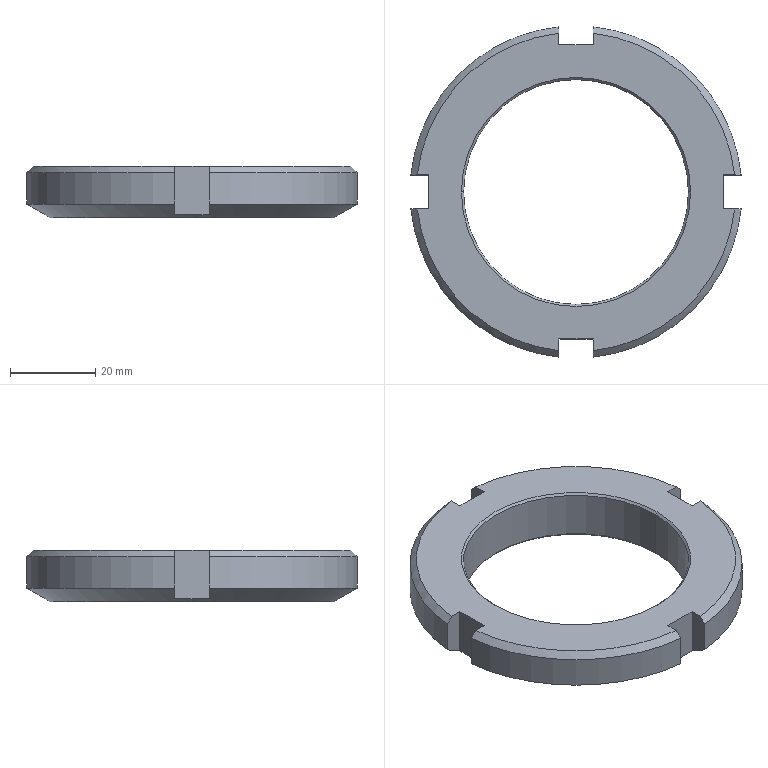Part | SolidWorks | features Chamfer 3, CirPattern 1, Cut 1, Extrusion 1 | 1 solid | 30 faces | box 77.589 x 77.589 x 12 mm | volume 27297 mm3 | plane 14 | cone 10 | cylinder 6 | commonest cylinder face diameters 78 x4 52.835 x2
STEP:
#1=CARTESIAN_POINT('',(-26.418,0.,11.5));
#2=VERTEX_POINT('',#1);
#3=CARTESIAN_POINT('',(26.418,0.,11.5));
#4=VERTEX_POINT('',#3);
#5=CARTESIAN_POINT('',(0.,0.,11.5));
#6=DIRECTION('',(0.,0.,1.));
#7=DIRECTION('',(1.,0.,0.));
#8=AXIS2_PLACEMENT_3D('',#5,#6,#7);
#9=CIRCLE('',#8,26.418);
#10=EDGE_CURVE('',#2,#4,#9,.T.);
#11=ORIENTED_EDGE('',*,*,#10,.F.);
#12=CARTESIAN_POINT('',(-26.918,0.,12.));
#13=VERTEX_POINT('',#12);
#14=CARTESIAN_POINT('',(-26.418,0.,11.5));
#15=DIRECTION('',(-0.7071,0.,0.7071));
#16=VECTOR('',#15,1000.);
#17=LINE('',#14,#16);
#18=EDGE_CURVE('',#2,#13,#17,.T.);
#19=ORIENTED_EDGE('',*,*,#18,.T.);
#20=CARTESIAN_POINT('',(26.918,0.,12.));
#21=VERTEX_POINT('',#20);
#22=CARTESIAN_POINT('',(0.,0.,12.));
#23=DIRECTION('',(0.,0.,-1.));
#24=DIRECTION('',(1.,0.,0.));
#25=AXIS2_PLACEMENT_3D('',#22,#23,#24);
#26=CIRCLE('',#25,26.918);
#27=EDGE_CURVE('',#21,#13,#26,.T.);
#28=ORIENTED_EDGE('',*,*,#27,.F.);
#29=CARTESIAN_POINT('',(26.418,0.,11.5));
#30=DIRECTION('',(0.7071,0.,0.7071));
#31=VECTOR('',#30,1000.);
#32=LINE('',#29,#31);
#33=EDGE_CURVE('',#4,#21,#32,.T.);
#34=ORIENTED_EDGE('',*,*,#33,.F.);
#35=EDGE_LOOP('',(#11,#19,#28,#34));
#36=FACE_OUTER_BOUND('',#35,.T.);
#37=CARTESIAN_POINT('',(0.,0.,11.5));
#38=DIRECTION('',(0.,0.,1.));
#39=DIRECTION('',(1.,0.,0.));
#40=AXIS2_PLACEMENT_3D('',#37,#38,#39);
#41=CONICAL_SURFACE('',#40,26.418,0.7854);
#42=ADVANCED_FACE('',(#36),#41,.F.);
#43=CARTESIAN_POINT('',(26.418,0.,0.5));
#44=VERTEX_POINT('',#43);
#45=CARTESIAN_POINT('',(-26.418,0.,0.5));
#46=VERTEX_POINT('',#45);
#47=CARTESIAN_POINT('',(0.,0.,0.5));
#48=DIRECTION('',(0.,0.,-1.));
#49=DIRECTION('',(1.,0.,0.));
#50=AXIS2_PLACEMENT_3D('',#47,#48,#49);
#51=CIRCLE('',#50,26.418);
#52=EDGE_CURVE('',#44,#46,#51,.T.);
#53=ORIENTED_EDGE('',*,*,#52,.F.);
#54=CARTESIAN_POINT('',(26.917,0.,0.));
#55=VERTEX_POINT('',#54);
#56=CARTESIAN_POINT('',(26.917,0.,0.));
#57=DIRECTION('',(0.7071,0.,-0.7071));
#58=VECTOR('',#57,1000.);
#59=LINE('',#56,#58);
#60=EDGE_CURVE('',#44,#55,#59,.T.);
#61=ORIENTED_EDGE('',*,*,#60,.T.);
#62=CARTESIAN_POINT('',(-26.917,0.,0.));
#63=VERTEX_POINT('',#62);
#64=CARTESIAN_POINT('',(0.,0.,0.));
#65=DIRECTION('',(0.,0.,1.));
#66=DIRECTION('',(1.,0.,0.));
#67=AXIS2_PLACEMENT_3D('',#64,#65,#66);
#68=CIRCLE('',#67,26.917);
#69=EDGE_CURVE('',#63,#55,#68,.T.);
#70=ORIENTED_EDGE('',*,*,#69,.F.);
#71=CARTESIAN_POINT('',(-26.917,0.,0.));
#72=DIRECTION('',(-0.7071,0.,-0.7071));
#73=VECTOR('',#72,1000.);
#74=LINE('',#71,#73);
#75=EDGE_CURVE('',#46,#63,#74,.T.);
#76=ORIENTED_EDGE('',*,*,#75,.F.);
#77=EDGE_LOOP('',(#53,#61,#70,#76));
#78=FACE_OUTER_BOUND('',#77,.T.);
#79=CARTESIAN_POINT('',(0.,0.,0.));
#80=DIRECTION('',(0.,0.,-1.));
#81=DIRECTION('',(-1.,0.,0.));
#82=AXIS2_PLACEMENT_3D('',#79,#80,#81);
#83=CONICAL_SURFACE('',#82,26.917,0.7854);
#84=ADVANCED_FACE('',(#78),#83,.F.);
#85=CARTESIAN_POINT('',(-33.5,0.,0.));
#86=VERTEX_POINT('',#85);
#87=CARTESIAN_POINT('',(33.5,0.,0.));
#88=VERTEX_POINT('',#87);
#89=CARTESIAN_POINT('',(0.,0.,0.));
#90=DIRECTION('',(0.,0.,-1.));
#91=DIRECTION('',(1.,0.,0.));
#92=AXIS2_PLACEMENT_3D('',#89,#90,#91);
#93=CIRCLE('',#92,33.5);
#94=EDGE_CURVE('',#86,#88,#93,.T.);
#95=ORIENTED_EDGE('',*,*,#94,.F.);
#96=CARTESIAN_POINT('',(-34.544,0.,0.6029));
#97=VERTEX_POINT('',#96);
#98=CARTESIAN_POINT('',(-39.,0.,3.175));
#99=DIRECTION('',(-0.866,0.,0.5));
#100=VECTOR('',#99,1000.);
#101=LINE('',#98,#100);
#102=EDGE_CURVE('',#86,#97,#101,.T.);
#103=ORIENTED_EDGE('',*,*,#102,.T.);
#104=CARTESIAN_POINT('',(-34.544,4.,0.7362));
#105=VERTEX_POINT('',#104);
#106=CARTESIAN_POINT('',(-34.544,4.,0.7362));
#107=CARTESIAN_POINT('',(-34.544,2.671,0.6479));
#108=CARTESIAN_POINT('',(-34.544,1.337,0.6029));
#109=CARTESIAN_POINT('',(-34.544,0.,0.6029));
#110=B_SPLINE_CURVE_WITH_KNOTS('',3,(#106,#107,#108,#109),.UNSPECIFIED.,.F.,.F.,(4,4),(0.01042,0.01441),.UNSPECIFIED.);
#111=EDGE_CURVE('',#105,#97,#110,.T.);
#112=ORIENTED_EDGE('',*,*,#111,.F.);
#113=CARTESIAN_POINT('',(-38.794,4.,3.175));
#114=VERTEX_POINT('',#113);
#115=CARTESIAN_POINT('',(-38.794,4.,3.175));
#116=CARTESIAN_POINT('',(-38.547,4.,3.033));
#117=CARTESIAN_POINT('',(-38.299,4.,2.891));
#118=CARTESIAN_POINT('',(-38.052,4.,2.749));
#119=CARTESIAN_POINT('',(-36.883,4.,2.078));
#120=CARTESIAN_POINT('',(-35.714,4.,1.407));
#121=CARTESIAN_POINT('',(-34.544,4.,0.7362));
#122=B_SPLINE_CURVE_WITH_KNOTS('',3,(#115,#116,#117,#118,#119,#120,#121),.UNSPECIFIED.,.F.,.F.,(4,3,4),(0.009232,0.01009,0.01413),.UNSPECIFIED.);
#123=EDGE_CURVE('',#114,#105,#122,.T.);
#124=ORIENTED_EDGE('',*,*,#123,.F.);
#125=CARTESIAN_POINT('',(-4.,38.794,3.175));
#126=VERTEX_POINT('',#125);
#127=CARTESIAN_POINT('',(0.,0.,3.175));
#128=DIRECTION('',(0.,0.,1.));
#129=DIRECTION('',(1.,0.,0.));
#130=AXIS2_PLACEMENT_3D('',#127,#128,#129);
#131=CIRCLE('',#130,39.);
#132=EDGE_CURVE('',#126,#114,#131,.T.);
#133=ORIENTED_EDGE('',*,*,#132,.F.);
#134=CARTESIAN_POINT('',(-4.,34.544,0.7362));
#135=VERTEX_POINT('',#134);
#136=CARTESIAN_POINT('',(-4.,34.544,0.7362));
#137=CARTESIAN_POINT('',(-4.,35.961,1.549));
#138=CARTESIAN_POINT('',(-4.,37.378,2.362));
#139=CARTESIAN_POINT('',(-4.,38.794,3.175));
#140=B_SPLINE_CURVE_WITH_KNOTS('',3,(#136,#137,#138,#139),.UNSPECIFIED.,.F.,.F.,(4,4),(0.009598,0.0145),.UNSPECIFIED.);
#141=EDGE_CURVE('',#135,#126,#140,.T.);
#142=ORIENTED_EDGE('',*,*,#141,.F.);
#143=CARTESIAN_POINT('',(4.,34.544,0.7362));
#144=VERTEX_POINT('',#143);
#145=CARTESIAN_POINT('',(4.,34.544,0.7362));
#146=CARTESIAN_POINT('',(2.674,34.544,0.6482));
#147=CARTESIAN_POINT('',(1.345,34.544,0.6032));
#148=CARTESIAN_POINT('',(-0.6558,34.544,0.6028));
#149=CARTESIAN_POINT('',(-1.324,34.544,0.6139));
#150=CARTESIAN_POINT('',(-2.661,34.544,0.6583));
#151=CARTESIAN_POINT('',(-3.332,34.544,0.6918));
#152=CARTESIAN_POINT('',(-4.,34.544,0.7362));
#153=B_SPLINE_CURVE_WITH_KNOTS('',3,(#145,#146,#147,#148,#149,#150,#151,#152),.UNSPECIFIED.,.F.,.F.,(4,2,2,4),(0.01042,0.0144,0.01639,0.01839),.UNSPECIFIED.);
#154=EDGE_CURVE('',#144,#135,#153,.T.);
#155=ORIENTED_EDGE('',*,*,#154,.F.);
#156=CARTESIAN_POINT('',(4.,38.794,3.175));
#157=VERTEX_POINT('',#156);
#158=CARTESIAN_POINT('',(4.,38.794,3.175));
#159=CARTESIAN_POINT('',(4.,37.378,2.362));
#160=CARTESIAN_POINT('',(4.,35.961,1.549));
#161=CARTESIAN_POINT('',(4.,34.544,0.7362));
#162=B_SPLINE_CURVE_WITH_KNOTS('',3,(#158,#159,#160,#161),.UNSPECIFIED.,.F.,.F.,(4,4),(0.005677,0.01058),.UNSPECIFIED.);
#163=EDGE_CURVE('',#157,#144,#162,.T.);
#164=ORIENTED_EDGE('',*,*,#163,.F.);
#165=CARTESIAN_POINT('',(38.794,4.,3.175));
#166=VERTEX_POINT('',#165);
#167=CARTESIAN_POINT('',(0.,0.,3.175));
#168=DIRECTION('',(0.,0.,1.));
#169=DIRECTION('',(1.,0.,0.));
#170=AXIS2_PLACEMENT_3D('',#167,#168,#169);
#171=CIRCLE('',#170,39.);
#172=EDGE_CURVE('',#166,#157,#171,.T.);
#173=ORIENTED_EDGE('',*,*,#172,.F.);
#174=CARTESIAN_POINT('',(34.544,4.,0.7362));
#175=VERTEX_POINT('',#174);
#176=CARTESIAN_POINT('',(34.544,4.,0.7362));
#177=CARTESIAN_POINT('',(35.961,4.,1.549));
#178=CARTESIAN_POINT('',(37.378,4.,2.362));
#179=CARTESIAN_POINT('',(38.794,4.,3.175));
#180=B_SPLINE_CURVE_WITH_KNOTS('',3,(#176,#177,#178,#179),.UNSPECIFIED.,.F.,.F.,(4,4),(0.009598,0.0145),.UNSPECIFIED.);
#181=EDGE_CURVE('',#175,#166,#180,.T.);
#182=ORIENTED_EDGE('',*,*,#181,.F.);
#183=CARTESIAN_POINT('',(34.544,0.,0.6029));
#184=VERTEX_POINT('',#183);
#185=CARTESIAN_POINT('',(34.544,0.,0.6029));
#186=CARTESIAN_POINT('',(34.544,1.337,0.6029));
#187=CARTESIAN_POINT('',(34.544,2.671,0.6479));
#188=CARTESIAN_POINT('',(34.544,4.,0.7362));
#189=B_SPLINE_CURVE_WITH_KNOTS('',3,(#185,#186,#187,#188),.UNSPECIFIED.,.F.,.F.,(4,4),(0.02044,0.02444),.UNSPECIFIED.);
#190=EDGE_CURVE('',#184,#175,#189,.T.);
#191=ORIENTED_EDGE('',*,*,#190,.F.);
#192=CARTESIAN_POINT('',(39.,0.,3.175));
#193=DIRECTION('',(0.866,0.,0.5));
#194=VECTOR('',#193,1000.);
#195=LINE('',#192,#194);
#196=EDGE_CURVE('',#88,#184,#195,.T.);
#197=ORIENTED_EDGE('',*,*,#196,.F.);
#198=EDGE_LOOP('',(#95,#103,#112,#124,#133,#142,#155,#164,#173,#182,#191,#197));
#199=FACE_OUTER_BOUND('',#198,.T.);
#200=CARTESIAN_POINT('',(0.,0.,3.175));
#201=DIRECTION('',(0.,0.,1.));
#202=DIRECTION('',(1.,0.,0.));
#203=AXIS2_PLACEMENT_3D('',#200,#201,#202);
#204=CONICAL_SURFACE('',#203,39.,1.047);
#205=ADVANCED_FACE('',(#199),#204,.T.);
#206=ORIENTED_EDGE('',*,*,#10,.T.);
#207=CARTESIAN_POINT('',(26.418,0.,12.));
#208=DIRECTION('',(0.,0.,-1.));
#209=VECTOR('',#208,1000.);
#210=LINE('',#207,#209);
#211=EDGE_CURVE('',#4,#44,#210,.T.);
#212=ORIENTED_EDGE('',*,*,#211,.T.);
#213=ORIENTED_EDGE('',*,*,#52,.T.);
#214=CARTESIAN_POINT('',(-26.418,0.,12.));
#215=DIRECTION('',(0.,0.,-1.));
#216=VECTOR('',#215,1000.);
#217=LINE('',#214,#216);
#218=EDGE_CURVE('',#2,#46,#217,.T.);
#219=ORIENTED_EDGE('',*,*,#218,.F.);
#220=EDGE_LOOP('',(#206,#212,#213,#219));
#221=FACE_OUTER_BOUND('',#220,.T.);
#222=CARTESIAN_POINT('',(0.,0.,12.));
#223=DIRECTION('',(0.,0.,-1.));
#224=DIRECTION('',(-1.,0.,0.));
#225=AXIS2_PLACEMENT_3D('',#222,#223,#224);
#226=CYLINDRICAL_SURFACE('',#225,26.418);
#227=ADVANCED_FACE('',(#221),#226,.F.);
#228=CARTESIAN_POINT('',(4.,38.794,10.5));
#229=VERTEX_POINT('',#228);
#230=CARTESIAN_POINT('',(38.794,4.,10.5));
#231=VERTEX_POINT('',#230);
#232=CARTESIAN_POINT('',(0.,0.,10.5));
#233=DIRECTION('',(0.,0.,-1.));
#234=DIRECTION('',(1.,0.,0.));
#235=AXIS2_PLACEMENT_3D('',#232,#233,#234);
#236=CIRCLE('',#235,39.);
#237=EDGE_CURVE('',#229,#231,#236,.T.);
#238=ORIENTED_EDGE('',*,*,#237,.T.);
#239=CARTESIAN_POINT('',(38.794,4.,0.));
#240=DIRECTION('',(0.,0.,1.));
#241=VECTOR('',#240,1000.);
#242=LINE('',#239,#241);
#243=EDGE_CURVE('',#166,#231,#242,.T.);
#244=ORIENTED_EDGE('',*,*,#243,.F.);
#245=ORIENTED_EDGE('',*,*,#172,.T.);
#246=CARTESIAN_POINT('',(4.,38.794,0.));
#247=DIRECTION('',(0.,0.,1.));
#248=VECTOR('',#247,1000.);
#249=LINE('',#246,#248);
#250=EDGE_CURVE('',#157,#229,#249,.T.);
#251=ORIENTED_EDGE('',*,*,#250,.T.);
#252=EDGE_LOOP('',(#238,#244,#245,#251));
#253=FACE_OUTER_BOUND('',#252,.T.);
#254=CARTESIAN_POINT('',(0.,0.,12.));
#255=DIRECTION('',(0.,0.,-1.));
#256=DIRECTION('',(-1.,0.,0.));
#257=AXIS2_PLACEMENT_3D('',#254,#255,#256);
#258=CYLINDRICAL_SURFACE('',#257,39.);
#259=ADVANCED_FACE('',(#253),#258,.T.);
#260=CARTESIAN_POINT('',(37.286,4.,12.));
#261=VERTEX_POINT('',#260);
#262=CARTESIAN_POINT('',(38.794,4.,10.5));
#263=CARTESIAN_POINT('',(38.402,4.,10.89));
#264=CARTESIAN_POINT('',(38.01,4.,11.28));
#265=CARTESIAN_POINT('',(37.618,4.,11.67));
#266=CARTESIAN_POINT('',(37.507,4.,11.78));
#267=CARTESIAN_POINT('',(37.397,4.,11.89));
#268=CARTESIAN_POINT('',(37.286,4.,12.));
#269=B_SPLINE_CURVE_WITH_KNOTS('',3,(#262,#263,#264,#265,#266,#267,#268),.UNSPECIFIED.,.F.,.F.,(4,3,4),(0.007216,0.008875,0.009344),.UNSPECIFIED.);
#270=EDGE_CURVE('',#231,#261,#269,.T.);
#271=ORIENTED_EDGE('',*,*,#270,.F.);
#272=ORIENTED_EDGE('',*,*,#237,.F.);
#273=CARTESIAN_POINT('',(4.,37.286,12.));
#274=VERTEX_POINT('',#273);
#275=CARTESIAN_POINT('',(4.,37.286,12.));
#276=CARTESIAN_POINT('',(4.,37.397,11.89));
#277=CARTESIAN_POINT('',(4.,37.507,11.78));
#278=CARTESIAN_POINT('',(4.,37.618,11.67));
#279=CARTESIAN_POINT('',(4.,38.01,11.28));
#280=CARTESIAN_POINT('',(4.,38.402,10.89));
#281=CARTESIAN_POINT('',(4.,38.794,10.5));
#282=B_SPLINE_CURVE_WITH_KNOTS('',3,(#275,#276,#277,#278,#279,#280,#281),.UNSPECIFIED.,.F.,.F.,(4,3,4),(0.008407,0.008875,0.01053),.UNSPECIFIED.);
#283=EDGE_CURVE('',#274,#229,#282,.T.);
#284=ORIENTED_EDGE('',*,*,#283,.F.);
#285=CARTESIAN_POINT('',(0.,0.,12.));
#286=DIRECTION('',(0.,0.,1.));
#287=DIRECTION('',(1.,0.,0.));
#288=AXIS2_PLACEMENT_3D('',#285,#286,#287);
#289=CIRCLE('',#288,37.5);
#290=EDGE_CURVE('',#261,#274,#289,.T.);
#291=ORIENTED_EDGE('',*,*,#290,.F.);
#292=EDGE_LOOP('',(#271,#272,#284,#291));
#293=FACE_OUTER_BOUND('',#292,.T.);
#294=CARTESIAN_POINT('',(0.,0.,12.));
#295=DIRECTION('',(0.,0.,-1.));
#296=DIRECTION('',(-1.,0.,0.));
#297=AXIS2_PLACEMENT_3D('',#294,#295,#296);
#298=CONICAL_SURFACE('',#297,37.5,0.7854);
#299=ADVANCED_FACE('',(#293),#298,.T.);
#300=CARTESIAN_POINT('',(-38.794,4.,10.5));
#301=VERTEX_POINT('',#300);
#302=CARTESIAN_POINT('',(-4.,38.794,10.5));
#303=VERTEX_POINT('',#302);
#304=CARTESIAN_POINT('',(0.,0.,10.5));
#305=DIRECTION('',(0.,0.,-1.));
#306=DIRECTION('',(1.,0.,0.));
#307=AXIS2_PLACEMENT_3D('',#304,#305,#306);
#308=CIRCLE('',#307,39.);
#309=EDGE_CURVE('',#301,#303,#308,.T.);
#310=ORIENTED_EDGE('',*,*,#309,.T.);
#311=CARTESIAN_POINT('',(-4.,38.794,0.));
#312=DIRECTION('',(0.,0.,1.));
#313=VECTOR('',#312,1000.);
#314=LINE('',#311,#313);
#315=EDGE_CURVE('',#126,#303,#314,.T.);
#316=ORIENTED_EDGE('',*,*,#315,.F.);
#317=ORIENTED_EDGE('',*,*,#132,.T.);
#318=CARTESIAN_POINT('',(-38.794,4.,0.));
#319=DIRECTION('',(0.,0.,1.));
#320=VECTOR('',#319,1000.);
#321=LINE('',#318,#320);
#322=EDGE_CURVE('',#114,#301,#321,.T.);
#323=ORIENTED_EDGE('',*,*,#322,.T.);
#324=EDGE_LOOP('',(#310,#316,#317,#323));
#325=FACE_OUTER_BOUND('',#324,.T.);
#326=CARTESIAN_POINT('',(0.,0.,12.));
#327=DIRECTION('',(0.,0.,-1.));
#328=DIRECTION('',(-1.,0.,0.));
#329=AXIS2_PLACEMENT_3D('',#326,#327,#328);
#330=CYLINDRICAL_SURFACE('',#329,39.);
#331=ADVANCED_FACE('',(#325),#330,.T.);
#332=CARTESIAN_POINT('',(-4.,37.286,12.));
#333=VERTEX_POINT('',#332);
#334=CARTESIAN_POINT('',(-4.,38.794,10.5));
#335=CARTESIAN_POINT('',(-4.,38.402,10.89));
#336=CARTESIAN_POINT('',(-4.,38.01,11.28));
#337=CARTESIAN_POINT('',(-4.,37.618,11.67));
#338=CARTESIAN_POINT('',(-4.,37.507,11.78));
#339=CARTESIAN_POINT('',(-4.,37.397,11.89));
#340=CARTESIAN_POINT('',(-4.,37.286,12.));
#341=B_SPLINE_CURVE_WITH_KNOTS('',3,(#334,#335,#336,#337,#338,#339,#340),.UNSPECIFIED.,.F.,.F.,(4,3,4),(0.007216,0.008875,0.009344),.UNSPECIFIED.);
#342=EDGE_CURVE('',#303,#333,#341,.T.);
#343=ORIENTED_EDGE('',*,*,#342,.F.);
#344=ORIENTED_EDGE('',*,*,#309,.F.);
#345=CARTESIAN_POINT('',(-37.286,4.,12.));
#346=VERTEX_POINT('',#345);
#347=CARTESIAN_POINT('',(-37.286,4.,12.));
#348=CARTESIAN_POINT('',(-37.575,4.,11.713));
#349=CARTESIAN_POINT('',(-37.864,4.,11.426));
#350=CARTESIAN_POINT('',(-38.152,4.,11.139));
#351=CARTESIAN_POINT('',(-38.366,4.,10.926));
#352=CARTESIAN_POINT('',(-38.58,4.,10.713));
#353=CARTESIAN_POINT('',(-38.794,4.,10.5));
#354=B_SPLINE_CURVE_WITH_KNOTS('',3,(#347,#348,#349,#350,#351,#352,#353),.UNSPECIFIED.,.F.,.F.,(4,3,4),(0.007654,0.008875,0.009781),.UNSPECIFIED.);
#355=EDGE_CURVE('',#346,#301,#354,.T.);
#356=ORIENTED_EDGE('',*,*,#355,.F.);
#357=CARTESIAN_POINT('',(0.,0.,12.));
#358=DIRECTION('',(0.,0.,1.));
#359=DIRECTION('',(1.,0.,0.));
#360=AXIS2_PLACEMENT_3D('',#357,#358,#359);
#361=CIRCLE('',#360,37.5);
#362=EDGE_CURVE('',#333,#346,#361,.T.);
#363=ORIENTED_EDGE('',*,*,#362,.F.);
#364=EDGE_LOOP('',(#343,#344,#356,#363));
#365=FACE_OUTER_BOUND('',#364,.T.);
#366=CARTESIAN_POINT('',(0.,0.,12.));
#367=DIRECTION('',(0.,0.,-1.));
#368=DIRECTION('',(-1.,0.,0.));
#369=AXIS2_PLACEMENT_3D('',#366,#367,#368);
#370=CONICAL_SURFACE('',#369,37.5,0.7854);
#371=ADVANCED_FACE('',(#365),#370,.T.);
#372=CARTESIAN_POINT('',(-4.,-38.794,10.5));
#373=VERTEX_POINT('',#372);
#374=CARTESIAN_POINT('',(-38.794,-4.,10.5));
#375=VERTEX_POINT('',#374);
#376=CARTESIAN_POINT('',(0.,0.,10.5));
#377=DIRECTION('',(0.,0.,-1.));
#378=DIRECTION('',(1.,0.,0.));
#379=AXIS2_PLACEMENT_3D('',#376,#377,#378);
#380=CIRCLE('',#379,39.);
#381=EDGE_CURVE('',#373,#375,#380,.T.);
#382=ORIENTED_EDGE('',*,*,#381,.T.);
#383=CARTESIAN_POINT('',(-38.794,-4.,3.175));
#384=VERTEX_POINT('',#383);
#385=CARTESIAN_POINT('',(-38.794,-4.,0.));
#386=DIRECTION('',(0.,0.,1.));
#387=VECTOR('',#386,1000.);
#388=LINE('',#385,#387);
#389=EDGE_CURVE('',#384,#375,#388,.T.);
#390=ORIENTED_EDGE('',*,*,#389,.F.);
#391=CARTESIAN_POINT('',(-4.,-38.794,3.175));
#392=VERTEX_POINT('',#391);
#393=CARTESIAN_POINT('',(0.,0.,3.175));
#394=DIRECTION('',(0.,0.,1.));
#395=DIRECTION('',(1.,0.,0.));
#396=AXIS2_PLACEMENT_3D('',#393,#394,#395);
#397=CIRCLE('',#396,39.);
#398=EDGE_CURVE('',#384,#392,#397,.T.);
#399=ORIENTED_EDGE('',*,*,#398,.T.);
#400=CARTESIAN_POINT('',(-4.,-38.794,0.));
#401=DIRECTION('',(0.,0.,1.));
#402=VECTOR('',#401,1000.);
#403=LINE('',#400,#402);
#404=EDGE_CURVE('',#392,#373,#403,.T.);
#405=ORIENTED_EDGE('',*,*,#404,.T.);
#406=EDGE_LOOP('',(#382,#390,#399,#405));
#407=FACE_OUTER_BOUND('',#406,.T.);
#408=CARTESIAN_POINT('',(0.,0.,12.));
#409=DIRECTION('',(0.,0.,-1.));
#410=DIRECTION('',(-1.,0.,0.));
#411=AXIS2_PLACEMENT_3D('',#408,#409,#410);
#412=CYLINDRICAL_SURFACE('',#411,39.);
#413=ADVANCED_FACE('',(#407),#412,.T.);
#414=CARTESIAN_POINT('',(-37.286,-4.,12.));
#415=VERTEX_POINT('',#414);
#416=CARTESIAN_POINT('',(-38.794,-4.,10.5));
#417=CARTESIAN_POINT('',(-38.58,-4.,10.713));
#418=CARTESIAN_POINT('',(-38.366,-4.,10.926));
#419=CARTESIAN_POINT('',(-38.152,-4.,11.139));
#420=CARTESIAN_POINT('',(-37.864,-4.,11.426));
#421=CARTESIAN_POINT('',(-37.575,-4.,11.713));
#422=CARTESIAN_POINT('',(-37.286,-4.,12.));
#423=B_SPLINE_CURVE_WITH_KNOTS('',3,(#416,#417,#418,#419,#420,#421,#422),.UNSPECIFIED.,.F.,.F.,(4,3,4),(0.00797,0.008875,0.0101),.UNSPECIFIED.);
#424=EDGE_CURVE('',#375,#415,#423,.T.);
#425=ORIENTED_EDGE('',*,*,#424,.F.);
#426=ORIENTED_EDGE('',*,*,#381,.F.);
#427=CARTESIAN_POINT('',(-4.,-37.286,12.));
#428=VERTEX_POINT('',#427);
#429=CARTESIAN_POINT('',(-4.,-37.286,12.));
#430=CARTESIAN_POINT('',(-4.,-37.575,11.713));
#431=CARTESIAN_POINT('',(-4.,-37.864,11.426));
#432=CARTESIAN_POINT('',(-4.,-38.152,11.139));
#433=CARTESIAN_POINT('',(-4.,-38.366,10.926));
#434=CARTESIAN_POINT('',(-4.,-38.58,10.713));
#435=CARTESIAN_POINT('',(-4.,-38.794,10.5));
#436=B_SPLINE_CURVE_WITH_KNOTS('',3,(#429,#430,#431,#432,#433,#434,#435),.UNSPECIFIED.,.F.,.F.,(4,3,4),(0.007654,0.008875,0.009781),.UNSPECIFIED.);
#437=EDGE_CURVE('',#428,#373,#436,.T.);
#438=ORIENTED_EDGE('',*,*,#437,.F.);
#439=CARTESIAN_POINT('',(0.,0.,12.));
#440=DIRECTION('',(0.,0.,1.));
#441=DIRECTION('',(1.,0.,0.));
#442=AXIS2_PLACEMENT_3D('',#439,#440,#441);
#443=CIRCLE('',#442,37.5);
#444=EDGE_CURVE('',#415,#428,#443,.T.);
#445=ORIENTED_EDGE('',*,*,#444,.F.);
#446=EDGE_LOOP('',(#425,#426,#438,#445));
#447=FACE_OUTER_BOUND('',#446,.T.);
#448=CARTESIAN_POINT('',(0.,0.,12.));
#449=DIRECTION('',(0.,0.,-1.));
#450=DIRECTION('',(-1.,0.,0.));
#451=AXIS2_PLACEMENT_3D('',#448,#449,#450);
#452=CONICAL_SURFACE('',#451,37.5,0.7854);
#453=ADVANCED_FACE('',(#447),#452,.T.);
#454=ORIENTED_EDGE('',*,*,#27,.T.);
#455=CARTESIAN_POINT('',(0.,0.,12.));
#456=DIRECTION('',(0.,0.,-1.));
#457=DIRECTION('',(1.,0.,0.));
#458=AXIS2_PLACEMENT_3D('',#455,#456,#457);
#459=CIRCLE('',#458,26.918);
#460=EDGE_CURVE('',#13,#21,#459,.T.);
#461=ORIENTED_EDGE('',*,*,#460,.T.);
#462=EDGE_LOOP('',(#454,#461));
#463=FACE_BOUND('',#462,.T.);
#464=CARTESIAN_POINT('',(34.544,4.,12.));
#465=VERTEX_POINT('',#464);
#466=CARTESIAN_POINT('',(34.544,4.,12.));
#467=DIRECTION('',(-1.,0.,0.));
#468=VECTOR('',#467,1000.);
#469=LINE('',#466,#468);
#470=EDGE_CURVE('',#261,#465,#469,.T.);
#471=ORIENTED_EDGE('',*,*,#470,.F.);
#472=ORIENTED_EDGE('',*,*,#290,.T.);
#473=CARTESIAN_POINT('',(4.,34.544,12.));
#474=VERTEX_POINT('',#473);
#475=CARTESIAN_POINT('',(4.,34.544,12.));
#476=DIRECTION('',(0.,1.,0.));
#477=VECTOR('',#476,1000.);
#478=LINE('',#475,#477);
#479=EDGE_CURVE('',#474,#274,#478,.T.);
#480=ORIENTED_EDGE('',*,*,#479,.F.);
#481=CARTESIAN_POINT('',(-4.,34.544,12.));
#482=VERTEX_POINT('',#481);
#483=CARTESIAN_POINT('',(4.,34.544,12.));
#484=DIRECTION('',(1.,0.,0.));
#485=VECTOR('',#484,1000.);
#486=LINE('',#483,#485);
#487=EDGE_CURVE('',#482,#474,#486,.T.);
#488=ORIENTED_EDGE('',*,*,#487,.F.);
#489=CARTESIAN_POINT('',(-4.,34.544,12.));
#490=DIRECTION('',(0.,-1.,0.));
#491=VECTOR('',#490,1000.);
#492=LINE('',#489,#491);
#493=EDGE_CURVE('',#333,#482,#492,.T.);
#494=ORIENTED_EDGE('',*,*,#493,.F.);
#495=ORIENTED_EDGE('',*,*,#362,.T.);
#496=CARTESIAN_POINT('',(-34.544,4.,12.));
#497=VERTEX_POINT('',#496);
#498=CARTESIAN_POINT('',(-34.544,4.,12.));
#499=DIRECTION('',(-1.,0.,0.));
#500=VECTOR('',#499,1000.);
#501=LINE('',#498,#500);
#502=EDGE_CURVE('',#497,#346,#501,.T.);
#503=ORIENTED_EDGE('',*,*,#502,.F.);
#504=CARTESIAN_POINT('',(-34.544,-4.,12.));
#505=VERTEX_POINT('',#504);
#506=CARTESIAN_POINT('',(-34.544,4.,12.));
#507=DIRECTION('',(0.,1.,0.));
#508=VECTOR('',#507,1000.);
#509=LINE('',#506,#508);
#510=EDGE_CURVE('',#505,#497,#509,.T.);
#511=ORIENTED_EDGE('',*,*,#510,.F.);
#512=CARTESIAN_POINT('',(-34.544,-4.,12.));
#513=DIRECTION('',(1.,0.,0.));
#514=VECTOR('',#513,1000.);
#515=LINE('',#512,#514);
#516=EDGE_CURVE('',#415,#505,#515,.T.);
#517=ORIENTED_EDGE('',*,*,#516,.F.);
#518=ORIENTED_EDGE('',*,*,#444,.T.);
#519=CARTESIAN_POINT('',(-4.,-34.544,12.));
#520=VERTEX_POINT('',#519);
#521=CARTESIAN_POINT('',(-4.,-34.544,12.));
#522=DIRECTION('',(0.,-1.,0.));
#523=VECTOR('',#522,1000.);
#524=LINE('',#521,#523);
#525=EDGE_CURVE('',#520,#428,#524,.T.);
#526=ORIENTED_EDGE('',*,*,#525,.F.);
#527=CARTESIAN_POINT('',(4.,-34.544,12.));
#528=VERTEX_POINT('',#527);
#529=CARTESIAN_POINT('',(-4.,-34.544,12.));
#530=DIRECTION('',(-1.,0.,0.));
#531=VECTOR('',#530,1000.);
#532=LINE('',#529,#531);
#533=EDGE_CURVE('',#528,#520,#532,.T.);
#534=ORIENTED_EDGE('',*,*,#533,.F.);
#535=CARTESIAN_POINT('',(4.,-37.286,12.));
#536=VERTEX_POINT('',#535);
#537=CARTESIAN_POINT('',(4.,-34.544,12.));
#538=DIRECTION('',(0.,1.,0.));
#539=VECTOR('',#538,1000.);
#540=LINE('',#537,#539);
#541=EDGE_CURVE('',#536,#528,#540,.T.);
#542=ORIENTED_EDGE('',*,*,#541,.F.);
#543=CARTESIAN_POINT('',(37.286,-4.,12.));
#544=VERTEX_POINT('',#543);
#545=CARTESIAN_POINT('',(0.,0.,12.));
#546=DIRECTION('',(0.,0.,1.));
#547=DIRECTION('',(1.,0.,0.));
#548=AXIS2_PLACEMENT_3D('',#545,#546,#547);
#549=CIRCLE('',#548,37.5);
#550=EDGE_CURVE('',#536,#544,#549,.T.);
#551=ORIENTED_EDGE('',*,*,#550,.T.);
#552=CARTESIAN_POINT('',(34.544,-4.,12.));
#553=VERTEX_POINT('',#552);
#554=CARTESIAN_POINT('',(34.544,-4.,12.));
#555=DIRECTION('',(1.,0.,0.));
#556=VECTOR('',#555,1000.);
#557=LINE('',#554,#556);
#558=EDGE_CURVE('',#553,#544,#557,.T.);
#559=ORIENTED_EDGE('',*,*,#558,.F.);
#560=CARTESIAN_POINT('',(34.544,-4.,12.));
#561=DIRECTION('',(0.,-1.,0.));
#562=VECTOR('',#561,1000.);
#563=LINE('',#560,#562);
#564=EDGE_CURVE('',#465,#553,#563,.T.);
#565=ORIENTED_EDGE('',*,*,#564,.F.);
#566=EDGE_LOOP('',(#471,#472,#480,#488,#494,#495,#503,#511,#517,#518,#526,#534,#542,#551,#559,#565));
#567=FACE_OUTER_BOUND('',#566,.T.);
#568=CARTESIAN_POINT('',(0.,0.,12.));
#569=DIRECTION('',(0.,0.,1.));
#570=DIRECTION('',(1.,0.,0.));
#571=AXIS2_PLACEMENT_3D('',#568,#569,#570);
#572=PLANE('',#571);
#573=ADVANCED_FACE('',(#463,#567),#572,.T.);
#574=ORIENTED_EDGE('',*,*,#69,.T.);
#575=CARTESIAN_POINT('',(0.,0.,0.));
#576=DIRECTION('',(0.,0.,1.));
#577=DIRECTION('',(1.,0.,0.));
#578=AXIS2_PLACEMENT_3D('',#575,#576,#577);
#579=CIRCLE('',#578,26.917);
#580=EDGE_CURVE('',#55,#63,#579,.T.);
#581=ORIENTED_EDGE('',*,*,#580,.T.);
#582=EDGE_LOOP('',(#574,#581));
#583=FACE_BOUND('',#582,.T.);
#584=CARTESIAN_POINT('',(0.,0.,0.));
#585=DIRECTION('',(0.,0.,-1.));
#586=DIRECTION('',(1.,0.,0.));
#587=AXIS2_PLACEMENT_3D('',#584,#585,#586);
#588=CIRCLE('',#587,33.5);
#589=EDGE_CURVE('',#88,#86,#588,.T.);
#590=ORIENTED_EDGE('',*,*,#589,.T.);
#591=ORIENTED_EDGE('',*,*,#94,.T.);
#592=EDGE_LOOP('',(#590,#591));
#593=FACE_OUTER_BOUND('',#592,.T.);
#594=CARTESIAN_POINT('',(0.,0.,0.));
#595=DIRECTION('',(0.,0.,1.));
#596=DIRECTION('',(1.,0.,0.));
#597=AXIS2_PLACEMENT_3D('',#594,#595,#596);
#598=PLANE('',#597);
#599=ADVANCED_FACE('',(#583,#593),#598,.F.);
#600=CARTESIAN_POINT('',(4.,-38.794,3.175));
#601=VERTEX_POINT('',#600);
#602=CARTESIAN_POINT('',(38.794,-4.,3.175));
#603=VERTEX_POINT('',#602);
#604=CARTESIAN_POINT('',(0.,0.,3.175));
#605=DIRECTION('',(0.,0.,1.));
#606=DIRECTION('',(1.,0.,0.));
#607=AXIS2_PLACEMENT_3D('',#604,#605,#606);
#608=CIRCLE('',#607,39.);
#609=EDGE_CURVE('',#601,#603,#608,.T.);
#610=ORIENTED_EDGE('',*,*,#609,.T.);
#611=CARTESIAN_POINT('',(38.794,-4.,10.5));
#612=VERTEX_POINT('',#611);
#613=CARTESIAN_POINT('',(38.794,-4.,0.));
#614=DIRECTION('',(0.,0.,1.));
#615=VECTOR('',#614,1000.);
#616=LINE('',#613,#615);
#617=EDGE_CURVE('',#603,#612,#616,.T.);
#618=ORIENTED_EDGE('',*,*,#617,.T.);
#619=CARTESIAN_POINT('',(4.,-38.794,10.5));
#620=VERTEX_POINT('',#619);
#621=CARTESIAN_POINT('',(0.,0.,10.5));
#622=DIRECTION('',(0.,0.,-1.));
#623=DIRECTION('',(1.,0.,0.));
#624=AXIS2_PLACEMENT_3D('',#621,#622,#623);
#625=CIRCLE('',#624,39.);
#626=EDGE_CURVE('',#612,#620,#625,.T.);
#627=ORIENTED_EDGE('',*,*,#626,.T.);
#628=CARTESIAN_POINT('',(4.,-38.794,0.));
#629=DIRECTION('',(0.,0.,1.));
#630=VECTOR('',#629,1000.);
#631=LINE('',#628,#630);
#632=EDGE_CURVE('',#601,#620,#631,.T.);
#633=ORIENTED_EDGE('',*,*,#632,.F.);
#634=EDGE_LOOP('',(#610,#618,#627,#633));
#635=FACE_OUTER_BOUND('',#634,.T.);
#636=CARTESIAN_POINT('',(0.,0.,12.));
#637=DIRECTION('',(0.,0.,-1.));
#638=DIRECTION('',(-1.,0.,0.));
#639=AXIS2_PLACEMENT_3D('',#636,#637,#638);
#640=CYLINDRICAL_SURFACE('',#639,39.);
#641=ADVANCED_FACE('',(#635),#640,.T.);
#642=ORIENTED_EDGE('',*,*,#211,.F.);
#643=CARTESIAN_POINT('',(0.,0.,11.5));
#644=DIRECTION('',(0.,0.,1.));
#645=DIRECTION('',(1.,0.,0.));
#646=AXIS2_PLACEMENT_3D('',#643,#644,#645);
#647=CIRCLE('',#646,26.418);
#648=EDGE_CURVE('',#4,#2,#647,.T.);
#649=ORIENTED_EDGE('',*,*,#648,.T.);
#650=ORIENTED_EDGE('',*,*,#218,.T.);
#651=CARTESIAN_POINT('',(0.,0.,0.5));
#652=DIRECTION('',(0.,0.,-1.));
#653=DIRECTION('',(1.,0.,0.));
#654=AXIS2_PLACEMENT_3D('',#651,#652,#653);
#655=CIRCLE('',#654,26.418);
#656=EDGE_CURVE('',#46,#44,#655,.T.);
#657=ORIENTED_EDGE('',*,*,#656,.T.);
#658=EDGE_LOOP('',(#642,#649,#650,#657));
#659=FACE_OUTER_BOUND('',#658,.T.);
#660=CARTESIAN_POINT('',(0.,0.,12.));
#661=DIRECTION('',(0.,0.,-1.));
#662=DIRECTION('',(-1.,0.,0.));
#663=AXIS2_PLACEMENT_3D('',#660,#661,#662);
#664=CYLINDRICAL_SURFACE('',#663,26.418);
#665=ADVANCED_FACE('',(#659),#664,.F.);
#666=CARTESIAN_POINT('',(37.286,-4.,12.));
#667=CARTESIAN_POINT('',(37.397,-4.,11.89));
#668=CARTESIAN_POINT('',(37.507,-4.,11.78));
#669=CARTESIAN_POINT('',(37.618,-4.,11.67));
#670=CARTESIAN_POINT('',(38.01,-4.,11.28));
#671=CARTESIAN_POINT('',(38.402,-4.,10.89));
#672=CARTESIAN_POINT('',(38.794,-4.,10.5));
#673=B_SPLINE_CURVE_WITH_KNOTS('',3,(#666,#667,#668,#669,#670,#671,#672),.UNSPECIFIED.,.F.,.F.,(4,3,4),(0.008407,0.008875,0.01053),.UNSPECIFIED.);
#674=EDGE_CURVE('',#544,#612,#673,.T.);
#675=ORIENTED_EDGE('',*,*,#674,.F.);
#676=ORIENTED_EDGE('',*,*,#550,.F.);
#677=CARTESIAN_POINT('',(4.,-38.794,10.5));
#678=CARTESIAN_POINT('',(4.,-38.58,10.713));
#679=CARTESIAN_POINT('',(4.,-38.366,10.926));
#680=CARTESIAN_POINT('',(4.,-38.152,11.139));
#681=CARTESIAN_POINT('',(4.,-37.864,11.426));
#682=CARTESIAN_POINT('',(4.,-37.575,11.713));
#683=CARTESIAN_POINT('',(4.,-37.286,12.));
#684=B_SPLINE_CURVE_WITH_KNOTS('',3,(#677,#678,#679,#680,#681,#682,#683),.UNSPECIFIED.,.F.,.F.,(4,3,4),(0.00797,0.008875,0.0101),.UNSPECIFIED.);
#685=EDGE_CURVE('',#620,#536,#684,.T.);
#686=ORIENTED_EDGE('',*,*,#685,.F.);
#687=ORIENTED_EDGE('',*,*,#626,.F.);
#688=EDGE_LOOP('',(#675,#676,#686,#687));
#689=FACE_OUTER_BOUND('',#688,.T.);
#690=CARTESIAN_POINT('',(0.,0.,12.));
#691=DIRECTION('',(0.,0.,-1.));
#692=DIRECTION('',(-1.,0.,0.));
#693=AXIS2_PLACEMENT_3D('',#690,#691,#692);
#694=CONICAL_SURFACE('',#693,37.5,0.7854);
#695=ADVANCED_FACE('',(#689),#694,.T.);
#696=ORIENTED_EDGE('',*,*,#102,.F.);
#697=ORIENTED_EDGE('',*,*,#589,.F.);
#698=ORIENTED_EDGE('',*,*,#196,.T.);
#699=CARTESIAN_POINT('',(34.544,-4.,0.7362));
#700=VERTEX_POINT('',#699);
#701=CARTESIAN_POINT('',(34.544,-4.,0.7362));
#702=CARTESIAN_POINT('',(34.544,-3.334,0.692));
#703=CARTESIAN_POINT('',(34.544,-2.665,0.6585));
#704=CARTESIAN_POINT('',(34.544,-1.331,0.614));
#705=CARTESIAN_POINT('',(34.544,-0.665,0.6029));
#706=CARTESIAN_POINT('',(34.544,0.,0.6029));
#707=B_SPLINE_CURVE_WITH_KNOTS('',3,(#701,#702,#703,#704,#705,#706),.UNSPECIFIED.,.F.,.F.,(4,2,4),(0.01646,0.01845,0.02044),.UNSPECIFIED.);
#708=EDGE_CURVE('',#700,#184,#707,.T.);
#709=ORIENTED_EDGE('',*,*,#708,.F.);
#710=CARTESIAN_POINT('',(38.794,-4.,3.175));
#711=CARTESIAN_POINT('',(37.378,-4.,2.362));
#712=CARTESIAN_POINT('',(35.961,-4.,1.549));
#713=CARTESIAN_POINT('',(34.544,-4.,0.7362));
#714=B_SPLINE_CURVE_WITH_KNOTS('',3,(#710,#711,#712,#713),.UNSPECIFIED.,.F.,.F.,(4,4),(0.005677,0.01058),.UNSPECIFIED.);
#715=EDGE_CURVE('',#603,#700,#714,.T.);
#716=ORIENTED_EDGE('',*,*,#715,.F.);
#717=ORIENTED_EDGE('',*,*,#609,.F.);
#718=CARTESIAN_POINT('',(4.,-34.544,0.7362));
#719=VERTEX_POINT('',#718);
#720=CARTESIAN_POINT('',(4.,-34.544,0.7362));
#721=CARTESIAN_POINT('',(4.,-35.714,1.407));
#722=CARTESIAN_POINT('',(4.,-36.883,2.078));
#723=CARTESIAN_POINT('',(4.,-38.052,2.749));
#724=CARTESIAN_POINT('',(4.,-38.299,2.891));
#725=CARTESIAN_POINT('',(4.,-38.547,3.033));
#726=CARTESIAN_POINT('',(4.,-38.794,3.175));
#727=B_SPLINE_CURVE_WITH_KNOTS('',3,(#720,#721,#722,#723,#724,#725,#726),.UNSPECIFIED.,.F.,.F.,(4,3,4),(0.006043,0.01009,0.01094),.UNSPECIFIED.);
#728=EDGE_CURVE('',#719,#601,#727,.T.);
#729=ORIENTED_EDGE('',*,*,#728,.F.);
#730=CARTESIAN_POINT('',(-4.,-34.544,0.7362));
#731=VERTEX_POINT('',#730);
#732=CARTESIAN_POINT('',(-4.,-34.544,0.7362));
#733=CARTESIAN_POINT('',(-3.332,-34.544,0.6918));
#734=CARTESIAN_POINT('',(-2.661,-34.544,0.6583));
#735=CARTESIAN_POINT('',(-1.324,-34.544,0.6139));
#736=CARTESIAN_POINT('',(-0.6558,-34.544,0.6028));
#737=CARTESIAN_POINT('',(1.345,-34.544,0.6032));
#738=CARTESIAN_POINT('',(2.674,-34.544,0.6482));
#739=CARTESIAN_POINT('',(4.,-34.544,0.7362));
#740=B_SPLINE_CURVE_WITH_KNOTS('',3,(#732,#733,#734,#735,#736,#737,#738,#739),.UNSPECIFIED.,.F.,.F.,(4,2,2,4),(0.01646,0.01845,0.02045,0.02444),.UNSPECIFIED.);
#741=EDGE_CURVE('',#731,#719,#740,.T.);
#742=ORIENTED_EDGE('',*,*,#741,.F.);
#743=CARTESIAN_POINT('',(-4.,-38.794,3.175));
#744=CARTESIAN_POINT('',(-4.,-38.547,3.033));
#745=CARTESIAN_POINT('',(-4.,-38.299,2.891));
#746=CARTESIAN_POINT('',(-4.,-38.052,2.749));
#747=CARTESIAN_POINT('',(-4.,-36.883,2.078));
#748=CARTESIAN_POINT('',(-4.,-35.714,1.407));
#749=CARTESIAN_POINT('',(-4.,-34.544,0.7362));
#750=B_SPLINE_CURVE_WITH_KNOTS('',3,(#743,#744,#745,#746,#747,#748,#749),.UNSPECIFIED.,.F.,.F.,(4,3,4),(0.009232,0.01009,0.01413),.UNSPECIFIED.);
#751=EDGE_CURVE('',#392,#731,#750,.T.);
#752=ORIENTED_EDGE('',*,*,#751,.F.);
#753=ORIENTED_EDGE('',*,*,#398,.F.);
#754=CARTESIAN_POINT('',(-34.544,-4.,0.7362));
#755=VERTEX_POINT('',#754);
#756=CARTESIAN_POINT('',(-34.544,-4.,0.7362));
#757=CARTESIAN_POINT('',(-35.714,-4.,1.407));
#758=CARTESIAN_POINT('',(-36.883,-4.,2.078));
#759=CARTESIAN_POINT('',(-38.052,-4.,2.749));
#760=CARTESIAN_POINT('',(-38.299,-4.,2.891));
#761=CARTESIAN_POINT('',(-38.547,-4.,3.033));
#762=CARTESIAN_POINT('',(-38.794,-4.,3.175));
#763=B_SPLINE_CURVE_WITH_KNOTS('',3,(#756,#757,#758,#759,#760,#761,#762),.UNSPECIFIED.,.F.,.F.,(4,3,4),(0.006043,0.01009,0.01094),.UNSPECIFIED.);
#764=EDGE_CURVE('',#755,#384,#763,.T.);
#765=ORIENTED_EDGE('',*,*,#764,.F.);
#766=CARTESIAN_POINT('',(-34.544,0.,0.6029));
#767=CARTESIAN_POINT('',(-34.544,-0.665,0.6029));
#768=CARTESIAN_POINT('',(-34.544,-1.331,0.614));
#769=CARTESIAN_POINT('',(-34.544,-2.665,0.6585));
#770=CARTESIAN_POINT('',(-34.544,-3.334,0.692));
#771=CARTESIAN_POINT('',(-34.544,-4.,0.7362));
#772=B_SPLINE_CURVE_WITH_KNOTS('',3,(#766,#767,#768,#769,#770,#771),.UNSPECIFIED.,.F.,.F.,(4,2,4),(0.01441,0.0164,0.01839),.UNSPECIFIED.);
#773=EDGE_CURVE('',#97,#755,#772,.T.);
#774=ORIENTED_EDGE('',*,*,#773,.F.);
#775=EDGE_LOOP('',(#696,#697,#698,#709,#716,#717,#729,#742,#752,#753,#765,#774));
#776=FACE_OUTER_BOUND('',#775,.T.);
#777=CARTESIAN_POINT('',(0.,0.,3.175));
#778=DIRECTION('',(0.,0.,1.));
#779=DIRECTION('',(1.,0.,0.));
#780=AXIS2_PLACEMENT_3D('',#777,#778,#779);
#781=CONICAL_SURFACE('',#780,39.,1.047);
#782=ADVANCED_FACE('',(#776),#781,.T.);
#783=ORIENTED_EDGE('',*,*,#741,.T.);
#784=CARTESIAN_POINT('',(4.,-34.544,0.));
#785=DIRECTION('',(0.,0.,1.));
#786=VECTOR('',#785,1000.);
#787=LINE('',#784,#786);
#788=EDGE_CURVE('',#719,#528,#787,.T.);
#789=ORIENTED_EDGE('',*,*,#788,.T.);
#790=ORIENTED_EDGE('',*,*,#533,.T.);
#791=CARTESIAN_POINT('',(-4.,-34.544,0.));
#792=DIRECTION('',(0.,0.,1.));
#793=VECTOR('',#792,1000.);
#794=LINE('',#791,#793);
#795=EDGE_CURVE('',#731,#520,#794,.T.);
#796=ORIENTED_EDGE('',*,*,#795,.F.);
#797=EDGE_LOOP('',(#783,#789,#790,#796));
#798=FACE_OUTER_BOUND('',#797,.T.);
#799=CARTESIAN_POINT('',(-4.,-34.544,0.));
#800=DIRECTION('',(0.,1.,0.));
#801=DIRECTION('',(0.,0.,1.));
#802=AXIS2_PLACEMENT_3D('',#799,#800,#801);
#803=PLANE('',#802);
#804=ADVANCED_FACE('',(#798),#803,.F.);
#805=ORIENTED_EDGE('',*,*,#685,.T.);
#806=ORIENTED_EDGE('',*,*,#541,.T.);
#807=ORIENTED_EDGE('',*,*,#788,.F.);
#808=ORIENTED_EDGE('',*,*,#728,.T.);
#809=ORIENTED_EDGE('',*,*,#632,.T.);
#810=EDGE_LOOP('',(#805,#806,#807,#808,#809));
#811=FACE_OUTER_BOUND('',#810,.T.);
#812=CARTESIAN_POINT('',(4.,-34.544,0.));
#813=DIRECTION('',(1.,0.,0.));
#814=DIRECTION('',(0.,1.,0.));
#815=AXIS2_PLACEMENT_3D('',#812,#813,#814);
#816=PLANE('',#815);
#817=ADVANCED_FACE('',(#811),#816,.F.);
#818=ORIENTED_EDGE('',*,*,#437,.T.);
#819=ORIENTED_EDGE('',*,*,#404,.F.);
#820=ORIENTED_EDGE('',*,*,#751,.T.);
#821=ORIENTED_EDGE('',*,*,#795,.T.);
#822=ORIENTED_EDGE('',*,*,#525,.T.);
#823=EDGE_LOOP('',(#818,#819,#820,#821,#822));
#824=FACE_OUTER_BOUND('',#823,.T.);
#825=CARTESIAN_POINT('',(-4.,-34.544,0.));
#826=DIRECTION('',(-1.,0.,0.));
#827=DIRECTION('',(0.,0.,1.));
#828=AXIS2_PLACEMENT_3D('',#825,#826,#827);
#829=PLANE('',#828);
#830=ADVANCED_FACE('',(#824),#829,.F.);
#831=ORIENTED_EDGE('',*,*,#111,.T.);
#832=ORIENTED_EDGE('',*,*,#773,.T.);
#833=CARTESIAN_POINT('',(-34.544,-4.,0.));
#834=DIRECTION('',(0.,0.,1.));
#835=VECTOR('',#834,1000.);
#836=LINE('',#833,#835);
#837=EDGE_CURVE('',#755,#505,#836,.T.);
#838=ORIENTED_EDGE('',*,*,#837,.T.);
#839=ORIENTED_EDGE('',*,*,#510,.T.);
#840=CARTESIAN_POINT('',(-34.544,4.,0.));
#841=DIRECTION('',(0.,0.,1.));
#842=VECTOR('',#841,1000.);
#843=LINE('',#840,#842);
#844=EDGE_CURVE('',#105,#497,#843,.T.);
#845=ORIENTED_EDGE('',*,*,#844,.F.);
#846=EDGE_LOOP('',(#831,#832,#838,#839,#845));
#847=FACE_OUTER_BOUND('',#846,.T.);
#848=CARTESIAN_POINT('',(-34.544,4.,0.));
#849=DIRECTION('',(1.,0.,0.));
#850=DIRECTION('',(0.,1.,0.));
#851=AXIS2_PLACEMENT_3D('',#848,#849,#850);
#852=PLANE('',#851);
#853=ADVANCED_FACE('',(#847),#852,.F.);
#854=ORIENTED_EDGE('',*,*,#424,.T.);
#855=ORIENTED_EDGE('',*,*,#516,.T.);
#856=ORIENTED_EDGE('',*,*,#837,.F.);
#857=ORIENTED_EDGE('',*,*,#764,.T.);
#858=ORIENTED_EDGE('',*,*,#389,.T.);
#859=EDGE_LOOP('',(#854,#855,#856,#857,#858));
#860=FACE_OUTER_BOUND('',#859,.T.);
#861=CARTESIAN_POINT('',(-34.544,-4.,0.));
#862=DIRECTION('',(0.,-1.,0.));
#863=DIRECTION('',(1.,0.,0.));
#864=AXIS2_PLACEMENT_3D('',#861,#862,#863);
#865=PLANE('',#864);
#866=ADVANCED_FACE('',(#860),#865,.F.);
#867=ORIENTED_EDGE('',*,*,#355,.T.);
#868=ORIENTED_EDGE('',*,*,#322,.F.);
#869=ORIENTED_EDGE('',*,*,#123,.T.);
#870=ORIENTED_EDGE('',*,*,#844,.T.);
#871=ORIENTED_EDGE('',*,*,#502,.T.);
#872=EDGE_LOOP('',(#867,#868,#869,#870,#871));
#873=FACE_OUTER_BOUND('',#872,.T.);
#874=CARTESIAN_POINT('',(-34.544,4.,0.));
#875=DIRECTION('',(0.,1.,0.));
#876=DIRECTION('',(-1.,0.,0.));
#877=AXIS2_PLACEMENT_3D('',#874,#875,#876);
#878=PLANE('',#877);
#879=ADVANCED_FACE('',(#873),#878,.F.);
#880=ORIENTED_EDGE('',*,*,#154,.T.);
#881=CARTESIAN_POINT('',(-4.,34.544,0.));
#882=DIRECTION('',(0.,0.,1.));
#883=VECTOR('',#882,1000.);
#884=LINE('',#881,#883);
#885=EDGE_CURVE('',#135,#482,#884,.T.);
#886=ORIENTED_EDGE('',*,*,#885,.T.);
#887=ORIENTED_EDGE('',*,*,#487,.T.);
#888=CARTESIAN_POINT('',(4.,34.544,0.));
#889=DIRECTION('',(0.,0.,1.));
#890=VECTOR('',#889,1000.);
#891=LINE('',#888,#890);
#892=EDGE_CURVE('',#144,#474,#891,.T.);
#893=ORIENTED_EDGE('',*,*,#892,.F.);
#894=EDGE_LOOP('',(#880,#886,#887,#893));
#895=FACE_OUTER_BOUND('',#894,.T.);
#896=CARTESIAN_POINT('',(4.,34.544,0.));
#897=DIRECTION('',(0.,-1.,0.));
#898=DIRECTION('',(1.,0.,0.));
#899=AXIS2_PLACEMENT_3D('',#896,#897,#898);
#900=PLANE('',#899);
#901=ADVANCED_FACE('',(#895),#900,.F.);
#902=ORIENTED_EDGE('',*,*,#342,.T.);
#903=ORIENTED_EDGE('',*,*,#493,.T.);
#904=ORIENTED_EDGE('',*,*,#885,.F.);
#905=ORIENTED_EDGE('',*,*,#141,.T.);
#906=ORIENTED_EDGE('',*,*,#315,.T.);
#907=EDGE_LOOP('',(#902,#903,#904,#905,#906));
#908=FACE_OUTER_BOUND('',#907,.T.);
#909=CARTESIAN_POINT('',(-4.,34.544,0.));
#910=DIRECTION('',(-1.,0.,0.));
#911=DIRECTION('',(0.,-1.,0.));
#912=AXIS2_PLACEMENT_3D('',#909,#910,#911);
#913=PLANE('',#912);
#914=ADVANCED_FACE('',(#908),#913,.F.);
#915=ORIENTED_EDGE('',*,*,#283,.T.);
#916=ORIENTED_EDGE('',*,*,#250,.F.);
#917=ORIENTED_EDGE('',*,*,#163,.T.);
#918=ORIENTED_EDGE('',*,*,#892,.T.);
#919=ORIENTED_EDGE('',*,*,#479,.T.);
#920=EDGE_LOOP('',(#915,#916,#917,#918,#919));
#921=FACE_OUTER_BOUND('',#920,.T.);
#922=CARTESIAN_POINT('',(4.,34.544,0.));
#923=DIRECTION('',(1.,0.,0.));
#924=DIRECTION('',(0.,1.,0.));
#925=AXIS2_PLACEMENT_3D('',#922,#923,#924);
#926=PLANE('',#925);
#927=ADVANCED_FACE('',(#921),#926,.F.);
#928=ORIENTED_EDGE('',*,*,#708,.T.);
#929=ORIENTED_EDGE('',*,*,#190,.T.);
#930=CARTESIAN_POINT('',(34.544,4.,0.));
#931=DIRECTION('',(0.,0.,1.));
#932=VECTOR('',#931,1000.);
#933=LINE('',#930,#932);
#934=EDGE_CURVE('',#175,#465,#933,.T.);
#935=ORIENTED_EDGE('',*,*,#934,.T.);
#936=ORIENTED_EDGE('',*,*,#564,.T.);
#937=CARTESIAN_POINT('',(34.544,-4.,0.));
#938=DIRECTION('',(0.,0.,1.));
#939=VECTOR('',#938,1000.);
#940=LINE('',#937,#939);
#941=EDGE_CURVE('',#700,#553,#940,.T.);
#942=ORIENTED_EDGE('',*,*,#941,.F.);
#943=EDGE_LOOP('',(#928,#929,#935,#936,#942));
#944=FACE_OUTER_BOUND('',#943,.T.);
#945=CARTESIAN_POINT('',(34.544,-4.,0.));
#946=DIRECTION('',(-1.,0.,0.));
#947=DIRECTION('',(0.,-1.,0.));
#948=AXIS2_PLACEMENT_3D('',#945,#946,#947);
#949=PLANE('',#948);
#950=ADVANCED_FACE('',(#944),#949,.F.);
#951=ORIENTED_EDGE('',*,*,#270,.T.);
#952=ORIENTED_EDGE('',*,*,#470,.T.);
#953=ORIENTED_EDGE('',*,*,#934,.F.);
#954=ORIENTED_EDGE('',*,*,#181,.T.);
#955=ORIENTED_EDGE('',*,*,#243,.T.);
#956=EDGE_LOOP('',(#951,#952,#953,#954,#955));
#957=FACE_OUTER_BOUND('',#956,.T.);
#958=CARTESIAN_POINT('',(34.544,4.,0.));
#959=DIRECTION('',(0.,1.,0.));
#960=DIRECTION('',(-1.,0.,0.));
#961=AXIS2_PLACEMENT_3D('',#958,#959,#960);
#962=PLANE('',#961);
#963=ADVANCED_FACE('',(#957),#962,.F.);
#964=ORIENTED_EDGE('',*,*,#674,.T.);
#965=ORIENTED_EDGE('',*,*,#617,.F.);
#966=ORIENTED_EDGE('',*,*,#715,.T.);
#967=ORIENTED_EDGE('',*,*,#941,.T.);
#968=ORIENTED_EDGE('',*,*,#558,.T.);
#969=EDGE_LOOP('',(#964,#965,#966,#967,#968));
#970=FACE_OUTER_BOUND('',#969,.T.);
#971=CARTESIAN_POINT('',(34.544,-4.,0.));
#972=DIRECTION('',(0.,-1.,0.));
#973=DIRECTION('',(1.,0.,0.));
#974=AXIS2_PLACEMENT_3D('',#971,#972,#973);
#975=PLANE('',#974);
#976=ADVANCED_FACE('',(#970),#975,.F.);
#977=ORIENTED_EDGE('',*,*,#60,.F.);
#978=ORIENTED_EDGE('',*,*,#656,.F.);
#979=ORIENTED_EDGE('',*,*,#75,.T.);
#980=ORIENTED_EDGE('',*,*,#580,.F.);
#981=EDGE_LOOP('',(#977,#978,#979,#980));
#982=FACE_OUTER_BOUND('',#981,.T.);
#983=CARTESIAN_POINT('',(0.,0.,0.));
#984=DIRECTION('',(0.,0.,-1.));
#985=DIRECTION('',(-1.,0.,0.));
#986=AXIS2_PLACEMENT_3D('',#983,#984,#985);
#987=CONICAL_SURFACE('',#986,26.917,0.7854);
#988=ADVANCED_FACE('',(#982),#987,.F.);
#989=ORIENTED_EDGE('',*,*,#18,.F.);
#990=ORIENTED_EDGE('',*,*,#648,.F.);
#991=ORIENTED_EDGE('',*,*,#33,.T.);
#992=ORIENTED_EDGE('',*,*,#460,.F.);
#993=EDGE_LOOP('',(#989,#990,#991,#992));
#994=FACE_OUTER_BOUND('',#993,.T.);
#995=CARTESIAN_POINT('',(0.,0.,11.5));
#996=DIRECTION('',(0.,0.,1.));
#997=DIRECTION('',(1.,0.,0.));
#998=AXIS2_PLACEMENT_3D('',#995,#996,#997);
#999=CONICAL_SURFACE('',#998,26.418,0.7854);
#1000=ADVANCED_FACE('',(#994),#999,.F.);
#1001=CLOSED_SHELL('',(#42,#84,#205,#227,#259,#299,#331,#371,#413,#453,#573,#599,#641,#665,#695,#782,#804,#817,#830,#853,#866,#879,#901,#914,#927,#950,#963,#976,#988,#1000));
#1002=MANIFOLD_SOLID_BREP('',#1001);
#1003=CARTESIAN_POINT('',(0.,0.,0.));
#1004=DIRECTION('',(0.,0.,1.));
#1005=DIRECTION('',(1.,0.,0.));
#1006=AXIS2_PLACEMENT_3D('',#1003,#1004,#1005);
#1007=(LENGTH_UNIT()NAMED_UNIT(*)SI_UNIT(.MILLI.,.METRE.));
#1008=UNCERTAINTY_MEASURE_WITH_UNIT(LENGTH_MEASURE(0.00001),#1007,'','');
#1009=(NAMED_UNIT(*)PLANE_ANGLE_UNIT()SI_UNIT($,.RADIAN.));
#1010=(NAMED_UNIT(*)SI_UNIT($,.STERADIAN.)SOLID_ANGLE_UNIT());
#1011=(GEOMETRIC_REPRESENTATION_CONTEXT(3)GLOBAL_UNCERTAINTY_ASSIGNED_CONTEXT((#1008))GLOBAL_UNIT_ASSIGNED_CONTEXT((#1007,#1009,#1010))REPRESENTATION_CONTEXT('',''));
#1012=ADVANCED_BREP_SHAPE_REPRESENTATION('',(#1002,#1006),#1011);